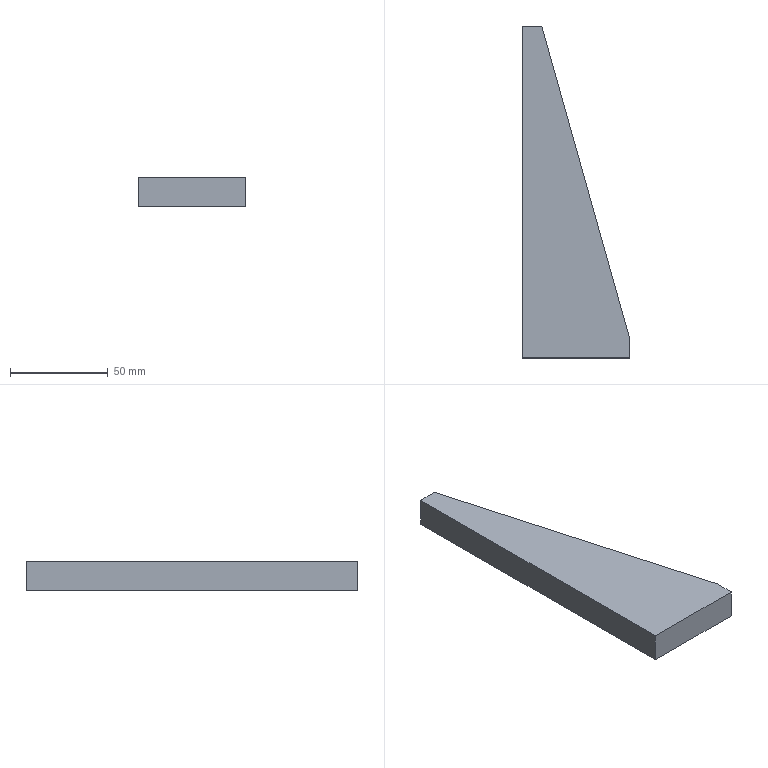Part | STEP file | 001-003-Shaft storage magazine rib plate | 1 solid | 7 faces | box 55 x 170 x 15 mm | volume 86250 mm3 | plane 7
STEP:
#1=CARTESIAN_POINT('',(0.,0.,0.));
#2=DIRECTION('',(0.,0.,1.));
#3=DIRECTION('',(1.,0.,0.));
#4=AXIS2_PLACEMENT_3D('',#1,#2,#3);
#5=CARTESIAN_POINT('',(27.5,-85.,0.));
#6=VERTEX_POINT('',#5);
#7=CARTESIAN_POINT('',(27.5,-75.,0.));
#8=VERTEX_POINT('',#7);
#9=CARTESIAN_POINT('',(27.5,-85.,0.));
#10=DIRECTION('',(0.,1.,0.));
#11=VECTOR('',#10,1.);
#12=LINE('',#9,#11);
#13=CARTESIAN_POINT('',(27.5,-85.,15.));
#14=DIRECTION('',(-1.,0.,0.));
#15=DIRECTION('',(0.,0.,1.));
#16=AXIS2_PLACEMENT_3D('',#13,#14,#15);
#17=PLANE('',#16);
#18=CARTESIAN_POINT('',(-15.,0.));
#19=DIRECTION('',(0.,1.));
#20=VECTOR('',#19,1.);
#21=LINE('',#18,#20);
#22=(GEOMETRIC_REPRESENTATION_CONTEXT(2)PARAMETRIC_REPRESENTATION_CONTEXT()REPRESENTATION_CONTEXT('',''));
#23=DEFINITIONAL_REPRESENTATION('',(#21),#22);
#24=PCURVE('',#17,#23);
#25=CARTESIAN_POINT('',(0.,0.,0.));
#26=DIRECTION('',(0.,0.,-1.));
#27=DIRECTION('',(-1.,0.,0.));
#28=AXIS2_PLACEMENT_3D('',#25,#26,#27);
#29=PLANE('',#28);
#30=CARTESIAN_POINT('',(-27.5,-85.));
#31=DIRECTION('',(0.,1.));
#32=VECTOR('',#31,1.);
#33=LINE('',#30,#32);
#34=(GEOMETRIC_REPRESENTATION_CONTEXT(2)PARAMETRIC_REPRESENTATION_CONTEXT()REPRESENTATION_CONTEXT('',''));
#35=DEFINITIONAL_REPRESENTATION('',(#33),#34);
#36=PCURVE('',#29,#35);
#37=SURFACE_CURVE('',#12,(#24,#36),.PCURVE_S1.);
#38=EDGE_CURVE('',#6,#8,#37,.T.);
#39=ORIENTED_EDGE('',*,*,#38,.T.);
#40=CARTESIAN_POINT('',(27.5,-75.,15.));
#41=VERTEX_POINT('',#40);
#42=CARTESIAN_POINT('',(27.5,-75.,15.));
#43=DIRECTION('',(0.,0.,1.));
#44=VECTOR('',#43,1.);
#45=LINE('',#42,#44);
#46=CARTESIAN_POINT('',(0.,10.));
#47=DIRECTION('',(1.,0.));
#48=VECTOR('',#47,1.);
#49=LINE('',#46,#48);
#50=(GEOMETRIC_REPRESENTATION_CONTEXT(2)PARAMETRIC_REPRESENTATION_CONTEXT()REPRESENTATION_CONTEXT('',''));
#51=DEFINITIONAL_REPRESENTATION('',(#49),#50);
#52=PCURVE('',#17,#51);
#53=CARTESIAN_POINT('',(-17.5,85.,15.));
#54=DIRECTION('',(-0.9627,-0.2707,0.));
#55=DIRECTION('',(0.,0.,-1.));
#56=AXIS2_PLACEMENT_3D('',#53,#54,#55);
#57=PLANE('',#56);
#58=CARTESIAN_POINT('',(0.,166.208));
#59=DIRECTION('',(-1.,0.));
#60=VECTOR('',#59,1.);
#61=LINE('',#58,#60);
#62=(GEOMETRIC_REPRESENTATION_CONTEXT(2)PARAMETRIC_REPRESENTATION_CONTEXT()REPRESENTATION_CONTEXT('',''));
#63=DEFINITIONAL_REPRESENTATION('',(#61),#62);
#64=PCURVE('',#57,#63);
#65=SURFACE_CURVE('',#45,(#52,#64),.PCURVE_S1.);
#66=EDGE_CURVE('',#8,#41,#65,.T.);
#67=ORIENTED_EDGE('',*,*,#66,.T.);
#68=CARTESIAN_POINT('',(27.5,-85.,15.));
#69=VERTEX_POINT('',#68);
#70=CARTESIAN_POINT('',(27.5,-85.,15.));
#71=DIRECTION('',(0.,1.,0.));
#72=VECTOR('',#71,1.);
#73=LINE('',#70,#72);
#74=CARTESIAN_POINT('',(0.,0.));
#75=DIRECTION('',(0.,1.));
#76=VECTOR('',#75,1.);
#77=LINE('',#74,#76);
#78=(GEOMETRIC_REPRESENTATION_CONTEXT(2)PARAMETRIC_REPRESENTATION_CONTEXT()REPRESENTATION_CONTEXT('',''));
#79=DEFINITIONAL_REPRESENTATION('',(#77),#78);
#80=PCURVE('',#17,#79);
#81=CARTESIAN_POINT('',(0.,0.,15.));
#82=DIRECTION('',(0.,0.,-1.));
#83=DIRECTION('',(-1.,0.,0.));
#84=AXIS2_PLACEMENT_3D('',#81,#82,#83);
#85=PLANE('',#84);
#86=CARTESIAN_POINT('',(-27.5,-85.));
#87=DIRECTION('',(0.,1.));
#88=VECTOR('',#87,1.);
#89=LINE('',#86,#88);
#90=(GEOMETRIC_REPRESENTATION_CONTEXT(2)PARAMETRIC_REPRESENTATION_CONTEXT()REPRESENTATION_CONTEXT('',''));
#91=DEFINITIONAL_REPRESENTATION('',(#89),#90);
#92=PCURVE('',#85,#91);
#93=SURFACE_CURVE('',#73,(#80,#92),.PCURVE_S1.);
#94=EDGE_CURVE('',#69,#41,#93,.T.);
#95=ORIENTED_EDGE('',*,*,#94,.F.);
#96=CARTESIAN_POINT('',(27.5,-85.,15.));
#97=DIRECTION('',(0.,0.,-1.));
#98=VECTOR('',#97,1.);
#99=LINE('',#96,#98);
#100=CARTESIAN_POINT('',(0.,0.));
#101=DIRECTION('',(-1.,0.));
#102=VECTOR('',#101,1.);
#103=LINE('',#100,#102);
#104=(GEOMETRIC_REPRESENTATION_CONTEXT(2)PARAMETRIC_REPRESENTATION_CONTEXT()REPRESENTATION_CONTEXT('',''));
#105=DEFINITIONAL_REPRESENTATION('',(#103),#104);
#106=PCURVE('',#17,#105);
#107=CARTESIAN_POINT('',(-27.5,-85.,15.));
#108=DIRECTION('',(0.,1.,0.));
#109=DIRECTION('',(0.,0.,1.));
#110=AXIS2_PLACEMENT_3D('',#107,#108,#109);
#111=PLANE('',#110);
#112=CARTESIAN_POINT('',(0.,55.));
#113=DIRECTION('',(-1.,0.));
#114=VECTOR('',#113,1.);
#115=LINE('',#112,#114);
#116=(GEOMETRIC_REPRESENTATION_CONTEXT(2)PARAMETRIC_REPRESENTATION_CONTEXT()REPRESENTATION_CONTEXT('',''));
#117=DEFINITIONAL_REPRESENTATION('',(#115),#116);
#118=PCURVE('',#111,#117);
#119=SURFACE_CURVE('',#99,(#106,#118),.PCURVE_S1.);
#120=EDGE_CURVE('',#69,#6,#119,.T.);
#121=ORIENTED_EDGE('',*,*,#120,.T.);
#122=EDGE_LOOP('',(#39,#67,#95,#121));
#123=FACE_BOUND('',#122,.T.);
#124=ADVANCED_FACE('',(#123),#17,.F.);
#125=CARTESIAN_POINT('',(-17.5,85.,15.));
#126=VERTEX_POINT('',#125);
#127=CARTESIAN_POINT('',(-27.5,85.,15.));
#128=VERTEX_POINT('',#127);
#129=CARTESIAN_POINT('',(-27.5,85.,15.));
#130=DIRECTION('',(-1.,0.,0.));
#131=VECTOR('',#130,1.);
#132=LINE('',#129,#131);
#133=CARTESIAN_POINT('',(-27.5,85.,15.));
#134=DIRECTION('',(0.,-1.,0.));
#135=DIRECTION('',(0.,0.,-1.));
#136=AXIS2_PLACEMENT_3D('',#133,#134,#135);
#137=PLANE('',#136);
#138=CARTESIAN_POINT('',(0.,0.));
#139=DIRECTION('',(0.,-1.));
#140=VECTOR('',#139,1.);
#141=LINE('',#138,#140);
#142=(GEOMETRIC_REPRESENTATION_CONTEXT(2)PARAMETRIC_REPRESENTATION_CONTEXT()REPRESENTATION_CONTEXT('',''));
#143=DEFINITIONAL_REPRESENTATION('',(#141),#142);
#144=PCURVE('',#137,#143);
#145=CARTESIAN_POINT('',(27.5,85.));
#146=DIRECTION('',(1.,0.));
#147=VECTOR('',#146,1.);
#148=LINE('',#145,#147);
#149=(GEOMETRIC_REPRESENTATION_CONTEXT(2)PARAMETRIC_REPRESENTATION_CONTEXT()REPRESENTATION_CONTEXT('',''));
#150=DEFINITIONAL_REPRESENTATION('',(#148),#149);
#151=PCURVE('',#85,#150);
#152=SURFACE_CURVE('',#132,(#144,#151),.PCURVE_S1.);
#153=EDGE_CURVE('',#126,#128,#152,.T.);
#154=ORIENTED_EDGE('',*,*,#153,.F.);
#155=CARTESIAN_POINT('',(-17.5,85.,0.));
#156=VERTEX_POINT('',#155);
#157=CARTESIAN_POINT('',(-17.5,85.,15.));
#158=DIRECTION('',(0.,0.,-1.));
#159=VECTOR('',#158,1.);
#160=LINE('',#157,#159);
#161=CARTESIAN_POINT('',(0.,10.));
#162=DIRECTION('',(1.,0.));
#163=VECTOR('',#162,1.);
#164=LINE('',#161,#163);
#165=(GEOMETRIC_REPRESENTATION_CONTEXT(2)PARAMETRIC_REPRESENTATION_CONTEXT()REPRESENTATION_CONTEXT('',''));
#166=DEFINITIONAL_REPRESENTATION('',(#164),#165);
#167=PCURVE('',#137,#166);
#168=CARTESIAN_POINT('',(0.,0.));
#169=DIRECTION('',(1.,0.));
#170=VECTOR('',#169,1.);
#171=LINE('',#168,#170);
#172=(GEOMETRIC_REPRESENTATION_CONTEXT(2)PARAMETRIC_REPRESENTATION_CONTEXT()REPRESENTATION_CONTEXT('',''));
#173=DEFINITIONAL_REPRESENTATION('',(#171),#172);
#174=PCURVE('',#57,#173);
#175=SURFACE_CURVE('',#160,(#167,#174),.PCURVE_S1.);
#176=EDGE_CURVE('',#126,#156,#175,.T.);
#177=ORIENTED_EDGE('',*,*,#176,.T.);
#178=CARTESIAN_POINT('',(-27.5,85.,0.));
#179=VERTEX_POINT('',#178);
#180=CARTESIAN_POINT('',(-27.5,85.,0.));
#181=DIRECTION('',(-1.,0.,0.));
#182=VECTOR('',#181,1.);
#183=LINE('',#180,#182);
#184=CARTESIAN_POINT('',(15.,0.));
#185=DIRECTION('',(0.,-1.));
#186=VECTOR('',#185,1.);
#187=LINE('',#184,#186);
#188=(GEOMETRIC_REPRESENTATION_CONTEXT(2)PARAMETRIC_REPRESENTATION_CONTEXT()REPRESENTATION_CONTEXT('',''));
#189=DEFINITIONAL_REPRESENTATION('',(#187),#188);
#190=PCURVE('',#137,#189);
#191=CARTESIAN_POINT('',(27.5,85.));
#192=DIRECTION('',(1.,0.));
#193=VECTOR('',#192,1.);
#194=LINE('',#191,#193);
#195=(GEOMETRIC_REPRESENTATION_CONTEXT(2)PARAMETRIC_REPRESENTATION_CONTEXT()REPRESENTATION_CONTEXT('',''));
#196=DEFINITIONAL_REPRESENTATION('',(#194),#195);
#197=PCURVE('',#29,#196);
#198=SURFACE_CURVE('',#183,(#190,#197),.PCURVE_S1.);
#199=EDGE_CURVE('',#156,#179,#198,.T.);
#200=ORIENTED_EDGE('',*,*,#199,.T.);
#201=CARTESIAN_POINT('',(-27.5,85.,15.));
#202=DIRECTION('',(0.,0.,-1.));
#203=VECTOR('',#202,1.);
#204=LINE('',#201,#203);
#205=CARTESIAN_POINT('',(0.,0.));
#206=DIRECTION('',(1.,0.));
#207=VECTOR('',#206,1.);
#208=LINE('',#205,#207);
#209=(GEOMETRIC_REPRESENTATION_CONTEXT(2)PARAMETRIC_REPRESENTATION_CONTEXT()REPRESENTATION_CONTEXT('',''));
#210=DEFINITIONAL_REPRESENTATION('',(#208),#209);
#211=PCURVE('',#137,#210);
#212=CARTESIAN_POINT('',(-27.5,-85.,15.));
#213=DIRECTION('',(1.,0.,0.));
#214=DIRECTION('',(0.,0.,-1.));
#215=AXIS2_PLACEMENT_3D('',#212,#213,#214);
#216=PLANE('',#215);
#217=CARTESIAN_POINT('',(0.,170.));
#218=DIRECTION('',(1.,0.));
#219=VECTOR('',#218,1.);
#220=LINE('',#217,#219);
#221=(GEOMETRIC_REPRESENTATION_CONTEXT(2)PARAMETRIC_REPRESENTATION_CONTEXT()REPRESENTATION_CONTEXT('',''));
#222=DEFINITIONAL_REPRESENTATION('',(#220),#221);
#223=PCURVE('',#216,#222);
#224=SURFACE_CURVE('',#204,(#211,#223),.PCURVE_S1.);
#225=EDGE_CURVE('',#128,#179,#224,.T.);
#226=ORIENTED_EDGE('',*,*,#225,.F.);
#227=EDGE_LOOP('',(#154,#177,#200,#226));
#228=FACE_BOUND('',#227,.T.);
#229=ADVANCED_FACE('',(#228),#137,.F.);
#230=CARTESIAN_POINT('',(-27.5,-85.,0.));
#231=VERTEX_POINT('',#230);
#232=CARTESIAN_POINT('',(-27.5,-85.,0.));
#233=DIRECTION('',(0.,-1.,0.));
#234=VECTOR('',#233,1.);
#235=LINE('',#232,#234);
#236=CARTESIAN_POINT('',(15.,0.));
#237=DIRECTION('',(0.,-1.));
#238=VECTOR('',#237,1.);
#239=LINE('',#236,#238);
#240=(GEOMETRIC_REPRESENTATION_CONTEXT(2)PARAMETRIC_REPRESENTATION_CONTEXT()REPRESENTATION_CONTEXT('',''));
#241=DEFINITIONAL_REPRESENTATION('',(#239),#240);
#242=PCURVE('',#216,#241);
#243=CARTESIAN_POINT('',(27.5,-85.));
#244=DIRECTION('',(0.,-1.));
#245=VECTOR('',#244,1.);
#246=LINE('',#243,#245);
#247=(GEOMETRIC_REPRESENTATION_CONTEXT(2)PARAMETRIC_REPRESENTATION_CONTEXT()REPRESENTATION_CONTEXT('',''));
#248=DEFINITIONAL_REPRESENTATION('',(#246),#247);
#249=PCURVE('',#29,#248);
#250=SURFACE_CURVE('',#235,(#242,#249),.PCURVE_S1.);
#251=EDGE_CURVE('',#179,#231,#250,.T.);
#252=ORIENTED_EDGE('',*,*,#251,.T.);
#253=CARTESIAN_POINT('',(-27.5,-85.,15.));
#254=VERTEX_POINT('',#253);
#255=CARTESIAN_POINT('',(-27.5,-85.,15.));
#256=DIRECTION('',(0.,0.,-1.));
#257=VECTOR('',#256,1.);
#258=LINE('',#255,#257);
#259=CARTESIAN_POINT('',(0.,0.));
#260=DIRECTION('',(1.,0.));
#261=VECTOR('',#260,1.);
#262=LINE('',#259,#261);
#263=(GEOMETRIC_REPRESENTATION_CONTEXT(2)PARAMETRIC_REPRESENTATION_CONTEXT()REPRESENTATION_CONTEXT('',''));
#264=DEFINITIONAL_REPRESENTATION('',(#262),#263);
#265=PCURVE('',#216,#264);
#266=CARTESIAN_POINT('',(0.,0.));
#267=DIRECTION('',(-1.,0.));
#268=VECTOR('',#267,1.);
#269=LINE('',#266,#268);
#270=(GEOMETRIC_REPRESENTATION_CONTEXT(2)PARAMETRIC_REPRESENTATION_CONTEXT()REPRESENTATION_CONTEXT('',''));
#271=DEFINITIONAL_REPRESENTATION('',(#269),#270);
#272=PCURVE('',#111,#271);
#273=SURFACE_CURVE('',#258,(#265,#272),.PCURVE_S1.);
#274=EDGE_CURVE('',#254,#231,#273,.T.);
#275=ORIENTED_EDGE('',*,*,#274,.F.);
#276=CARTESIAN_POINT('',(-27.5,-85.,15.));
#277=DIRECTION('',(0.,-1.,0.));
#278=VECTOR('',#277,1.);
#279=LINE('',#276,#278);
#280=CARTESIAN_POINT('',(0.,0.));
#281=DIRECTION('',(0.,-1.));
#282=VECTOR('',#281,1.);
#283=LINE('',#280,#282);
#284=(GEOMETRIC_REPRESENTATION_CONTEXT(2)PARAMETRIC_REPRESENTATION_CONTEXT()REPRESENTATION_CONTEXT('',''));
#285=DEFINITIONAL_REPRESENTATION('',(#283),#284);
#286=PCURVE('',#216,#285);
#287=CARTESIAN_POINT('',(27.5,-85.));
#288=DIRECTION('',(0.,-1.));
#289=VECTOR('',#288,1.);
#290=LINE('',#287,#289);
#291=(GEOMETRIC_REPRESENTATION_CONTEXT(2)PARAMETRIC_REPRESENTATION_CONTEXT()REPRESENTATION_CONTEXT('',''));
#292=DEFINITIONAL_REPRESENTATION('',(#290),#291);
#293=PCURVE('',#85,#292);
#294=SURFACE_CURVE('',#279,(#286,#293),.PCURVE_S1.);
#295=EDGE_CURVE('',#128,#254,#294,.T.);
#296=ORIENTED_EDGE('',*,*,#295,.F.);
#297=ORIENTED_EDGE('',*,*,#225,.T.);
#298=EDGE_LOOP('',(#252,#275,#296,#297));
#299=FACE_BOUND('',#298,.T.);
#300=ADVANCED_FACE('',(#299),#216,.F.);
#301=CARTESIAN_POINT('',(-27.5,-85.,0.));
#302=DIRECTION('',(1.,0.,0.));
#303=VECTOR('',#302,1.);
#304=LINE('',#301,#303);
#305=CARTESIAN_POINT('',(-15.,0.));
#306=DIRECTION('',(0.,1.));
#307=VECTOR('',#306,1.);
#308=LINE('',#305,#307);
#309=(GEOMETRIC_REPRESENTATION_CONTEXT(2)PARAMETRIC_REPRESENTATION_CONTEXT()REPRESENTATION_CONTEXT('',''));
#310=DEFINITIONAL_REPRESENTATION('',(#308),#309);
#311=PCURVE('',#111,#310);
#312=CARTESIAN_POINT('',(27.5,-85.));
#313=DIRECTION('',(-1.,0.));
#314=VECTOR('',#313,1.);
#315=LINE('',#312,#314);
#316=(GEOMETRIC_REPRESENTATION_CONTEXT(2)PARAMETRIC_REPRESENTATION_CONTEXT()REPRESENTATION_CONTEXT('',''));
#317=DEFINITIONAL_REPRESENTATION('',(#315),#316);
#318=PCURVE('',#29,#317);
#319=SURFACE_CURVE('',#304,(#311,#318),.PCURVE_S1.);
#320=EDGE_CURVE('',#231,#6,#319,.T.);
#321=ORIENTED_EDGE('',*,*,#320,.T.);
#322=ORIENTED_EDGE('',*,*,#120,.F.);
#323=CARTESIAN_POINT('',(-27.5,-85.,15.));
#324=DIRECTION('',(1.,0.,0.));
#325=VECTOR('',#324,1.);
#326=LINE('',#323,#325);
#327=CARTESIAN_POINT('',(0.,0.));
#328=DIRECTION('',(0.,1.));
#329=VECTOR('',#328,1.);
#330=LINE('',#327,#329);
#331=(GEOMETRIC_REPRESENTATION_CONTEXT(2)PARAMETRIC_REPRESENTATION_CONTEXT()REPRESENTATION_CONTEXT('',''));
#332=DEFINITIONAL_REPRESENTATION('',(#330),#331);
#333=PCURVE('',#111,#332);
#334=CARTESIAN_POINT('',(27.5,-85.));
#335=DIRECTION('',(-1.,0.));
#336=VECTOR('',#335,1.);
#337=LINE('',#334,#336);
#338=(GEOMETRIC_REPRESENTATION_CONTEXT(2)PARAMETRIC_REPRESENTATION_CONTEXT()REPRESENTATION_CONTEXT('',''));
#339=DEFINITIONAL_REPRESENTATION('',(#337),#338);
#340=PCURVE('',#85,#339);
#341=SURFACE_CURVE('',#326,(#333,#340),.PCURVE_S1.);
#342=EDGE_CURVE('',#254,#69,#341,.T.);
#343=ORIENTED_EDGE('',*,*,#342,.F.);
#344=ORIENTED_EDGE('',*,*,#274,.T.);
#345=EDGE_LOOP('',(#321,#322,#343,#344));
#346=FACE_BOUND('',#345,.T.);
#347=ADVANCED_FACE('',(#346),#111,.F.);
#348=ORIENTED_EDGE('',*,*,#94,.T.);
#349=CARTESIAN_POINT('',(-17.5,85.,15.));
#350=DIRECTION('',(-0.2707,0.9627,0.));
#351=VECTOR('',#350,1.);
#352=LINE('',#349,#351);
#353=CARTESIAN_POINT('',(17.5,85.));
#354=DIRECTION('',(0.2707,0.9627));
#355=VECTOR('',#354,1.);
#356=LINE('',#353,#355);
#357=(GEOMETRIC_REPRESENTATION_CONTEXT(2)PARAMETRIC_REPRESENTATION_CONTEXT()REPRESENTATION_CONTEXT('',''));
#358=DEFINITIONAL_REPRESENTATION('',(#356),#357);
#359=PCURVE('',#85,#358);
#360=CARTESIAN_POINT('',(0.,0.));
#361=DIRECTION('',(0.,-1.));
#362=VECTOR('',#361,1.);
#363=LINE('',#360,#362);
#364=(GEOMETRIC_REPRESENTATION_CONTEXT(2)PARAMETRIC_REPRESENTATION_CONTEXT()REPRESENTATION_CONTEXT('',''));
#365=DEFINITIONAL_REPRESENTATION('',(#363),#364);
#366=PCURVE('',#57,#365);
#367=SURFACE_CURVE('',#352,(#359,#366),.PCURVE_S1.);
#368=EDGE_CURVE('',#41,#126,#367,.T.);
#369=ORIENTED_EDGE('',*,*,#368,.T.);
#370=ORIENTED_EDGE('',*,*,#153,.T.);
#371=ORIENTED_EDGE('',*,*,#295,.T.);
#372=ORIENTED_EDGE('',*,*,#342,.T.);
#373=EDGE_LOOP('',(#348,#369,#370,#371,#372));
#374=FACE_BOUND('',#373,.T.);
#375=ADVANCED_FACE('',(#374),#85,.F.);
#376=ORIENTED_EDGE('',*,*,#199,.F.);
#377=CARTESIAN_POINT('',(5.937,1.67,0.));
#378=DIRECTION('',(0.2707,-0.9627,0.));
#379=VECTOR('',#378,1.);
#380=LINE('',#377,#379);
#381=CARTESIAN_POINT('',(-5.937,1.67));
#382=DIRECTION('',(-0.2707,-0.9627));
#383=VECTOR('',#382,1.);
#384=LINE('',#381,#383);
#385=(GEOMETRIC_REPRESENTATION_CONTEXT(2)PARAMETRIC_REPRESENTATION_CONTEXT()REPRESENTATION_CONTEXT('',''));
#386=DEFINITIONAL_REPRESENTATION('',(#384),#385);
#387=PCURVE('',#29,#386);
#388=CARTESIAN_POINT('',(15.,86.563));
#389=DIRECTION('',(0.,1.));
#390=VECTOR('',#389,1.);
#391=LINE('',#388,#390);
#392=(GEOMETRIC_REPRESENTATION_CONTEXT(2)PARAMETRIC_REPRESENTATION_CONTEXT()REPRESENTATION_CONTEXT('',''));
#393=DEFINITIONAL_REPRESENTATION('',(#391),#392);
#394=PCURVE('',#57,#393);
#395=SURFACE_CURVE('',#380,(#387,#394),.PCURVE_S1.);
#396=EDGE_CURVE('',#156,#8,#395,.T.);
#397=ORIENTED_EDGE('',*,*,#396,.T.);
#398=ORIENTED_EDGE('',*,*,#38,.F.);
#399=ORIENTED_EDGE('',*,*,#320,.F.);
#400=ORIENTED_EDGE('',*,*,#251,.F.);
#401=EDGE_LOOP('',(#376,#397,#398,#399,#400));
#402=FACE_BOUND('',#401,.T.);
#403=ADVANCED_FACE('',(#402),#29,.T.);
#404=ORIENTED_EDGE('',*,*,#368,.F.);
#405=ORIENTED_EDGE('',*,*,#66,.F.);
#406=ORIENTED_EDGE('',*,*,#396,.F.);
#407=ORIENTED_EDGE('',*,*,#176,.F.);
#408=EDGE_LOOP('',(#404,#405,#406,#407));
#409=FACE_BOUND('',#408,.T.);
#410=ADVANCED_FACE('',(#409),#57,.F.);
#411=CLOSED_SHELL('',(#124,#229,#300,#347,#375,#403,#410));
#412=MANIFOLD_SOLID_BREP('',#411);
#413=(LENGTH_UNIT()NAMED_UNIT(*)SI_UNIT(.MILLI.,.METRE.));
#414=UNCERTAINTY_MEASURE_WITH_UNIT(LENGTH_MEASURE(0.0000001),#413,'','');
#415=(NAMED_UNIT(*)PLANE_ANGLE_UNIT()SI_UNIT($,.RADIAN.));
#416=(NAMED_UNIT(*)SI_UNIT($,.STERADIAN.)SOLID_ANGLE_UNIT());
#417=(GEOMETRIC_REPRESENTATION_CONTEXT(3)GLOBAL_UNCERTAINTY_ASSIGNED_CONTEXT((#414))GLOBAL_UNIT_ASSIGNED_CONTEXT((#413,#415,#416))REPRESENTATION_CONTEXT('',''));
#418=ADVANCED_BREP_SHAPE_REPRESENTATION('',(#4,#412),#417);